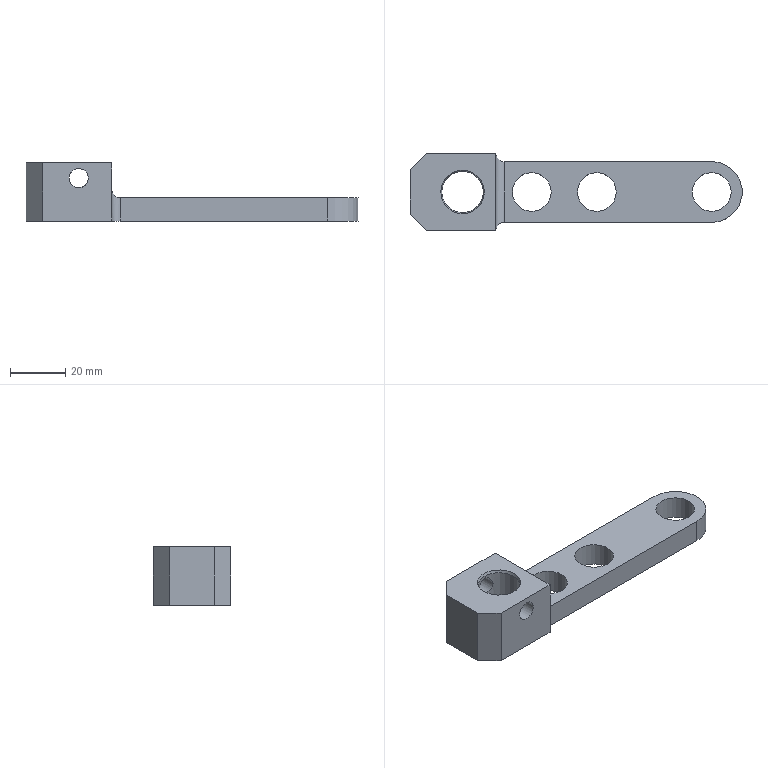NC program | NX | posted with a generic post | part box 120 x 28 x 21 mm
Lines 1651 to 1970 of 1970:
(ZLEVEL_PROFILE_STEEP , TOOL : 5R0.5)
N3246 T07 M6
N3248 G53
N3250 G17 G0 G90 X-41.022 Y-0.016 B0. C0. S4500 M3
N3252 G43 Z20. H7
N3254 Z1.172
N3256 G94 G1 Z0.172 F1000.
N3258 X-43.402 Y-1.627
N3260 G3 X-41.002 Y-4.027 R2.4
N3262 X-36.977 Y-0.003 R4.024
N3264 X-41.002 Y-4.027 R-4.024
N3266 G1 X-40.719 Y-4.002 Z0.157
N3268 X-40.435 Y-3.977 Z0.142
N3270 G3 X-41.002 Y-4.017 R-4.014
N3272 G1 X-40.719 Y-3.991 Z0.127
N3274 X-40.436 Y-3.964 Z0.112
N3276 G3 X-41.002 Y-4.004 R-4.002
N3278 G1 X-40.719 Y-3.98 Z0.097
N3280 X-40.436 Y-3.952 Z0.082
N3282 G3 X-41.002 Y-3.992 R-3.99
N3284 G1 X-40.719 Y-3.969 Z0.067
N3286 X-40.436 Y-3.939 Z0.052
N3288 G3 X-41.002 Y-3.979 R-3.979
N3290 G1 X-40.718 Y-3.959 Z0.037
N3292 X-40.436 Y-3.926 Z0.022
N3294 G3 X-41.002 Y-3.966 R-3.966
N3296 G1 X-40.718 Y-3.948 Z0.007
N3298 X-40.434 Y-3.924 Z-0.007
N3300 G3 X-41.002 Y-3.964 R-3.964
N3302 G1 X-40.719 Y-3.937 Z-0.022
N3304 X-40.437 Y-3.905 Z-0.037
N3306 G3 X-41.002 Y-3.946 R-3.946
N3308 G1 X-40.718 Y-3.926 Z-0.052
N3310 X-40.435 Y-3.896 Z-0.067
N3312 G3 X-41.002 Y-3.936 R-3.936
N3314 G1 X-40.718 Y-3.916 Z-0.082
N3316 X-40.436 Y-3.883 Z-0.097
N3318 G3 X-41.002 Y-3.924 R-3.924
N3320 G1 X-40.718 Y-3.906 Z-0.112
N3322 X-40.436 Y-3.873 Z-0.127
N3324 G3 X-41.002 Y-3.914 R-3.914
N3326 G1 X-40.718 Y-3.896 Z-0.142
N3328 X-40.435 Y-3.863 Z-0.157
N3330 G3 X-41.002 Y-3.904 R-3.904
N3332 G1 X-40.718 Y-3.886 Z-0.172
N3334 X-40.435 Y-3.854 Z-0.187
N3336 G3 X-41.002 Y-3.895 R-3.894
N3338 G1 X-40.718 Y-3.876 Z-0.201
N3340 X-40.436 Y-3.842 Z-0.216
N3342 G3 X-41.002 Y-3.884 R-3.883
N3344 G1 X-40.718 Y-3.867 Z-0.231
N3346 X-40.436 Y-3.833 Z-0.246
N3348 G3 X-41.002 Y-3.874 R-3.873
N3350 G1 X-40.718 Y-3.857 Z-0.261
N3352 X-40.436 Y-3.82 Z-0.276
N3354 G3 X-41.002 Y-3.861 R-3.861
N3356 G1 X-40.718 Y-3.848 Z-0.291
N3358 X-40.436 Y-3.81 Z-0.306
N3360 G3 X-41.002 Y-3.852 R-3.852
N3362 G1 X-40.718 Y-3.838 Z-0.321
N3364 X-40.436 Y-3.8 Z-0.336
N3366 G3 X-41.002 Y-3.842 R-3.842
N3368 G1 X-40.717 Y-3.827 Z-0.351
N3370 X-40.433 Y-3.807 Z-0.366
N3372 G3 X-38.622 Y-3.01 R4.394
N3374 G1 X-38.612 Y-3.021
N3376 G3 X-37.201 Y-0.629 R3.851
N3378 X-37.201 Y0.629 R6.692
N3380 G1 X-37.218 Y0.724
N3382 G3 X-41.357 Y3.837 R3.921
N3384 X-43.396 Y2.996 R4.255
N3386 X-44.6 Y1.289 R3.498
N3388 G1 X-44.783 Y0.721
N3390 X-44.799 Y0.629
N3392 G3 X-44.799 Y-0.629 R5.812
N3394 X-43.393 Y-3.017 R3.851
N3396 G1 X-43.383 Y-3.006
N3398 G3 X-41.002 Y-3.849 R3.987
N3400 G1 X-40.718 Y-3.835 Z-0.381
N3402 X-40.437 Y-3.798 Z-0.396
N3404 G3 X-38.276 Y2.707 R3.84
N3406 G1 X-38.997 Y3.304
N3408 G3 X-40.396 Y3.792 R6.376
N3410 X-43.265 Y3.1 R3.84
N3412 G1 X-43.257 Y3.089
N3414 X-43.347 Y3.022
N3416 G3 X-44.701 Y0.966 R3.747
N3418 G1 X-44.746 Y0.776
N3420 X-44.767 Y0.744
N3422 G3 X-43.385 Y-3.009 R3.84
N3424 G1 X-43.259 Y-3.092
N3426 X-42.982 Y-3.289
N3428 G3 X-41.002 Y-3.84 R3.84
N3430 G1 X-40.718 Y-3.824 Z-0.41
N3432 X-40.436 Y-3.787 Z-0.425
N3434 G3 X-39.161 Y-3.359 R3.829
N3436 G1 X-38.66 Y-3.016
N3438 X-38.626 Y-3.004
N3440 G3 X-37.417 Y-1.352 R3.829
N3442 G1 X-37.243 Y-0.741
N3444 G3 X-38.095 Y2.495 R3.829
N3446 G1 X-38.515 Y2.913
N3448 X-38.59 Y2.976
N3450 X-38.646 Y3.006
N3452 X-38.741 Y3.092
N3454 G3 X-39.655 Y3.585 R3.829
N3456 X-40.398 Y3.782 R28.134
N3458 X-43.259 Y3.092 R3.829
N3460 G1 X-43.276 Y3.064
N3462 X-43.387 Y2.98
N3464 G3 X-44.695 Y0.947 R3.792
N3466 G2 X-44.757 Y0.741 R2.485
N3468 G3 X-43.182 Y-3.146 R3.829
N3470 G1 X-42.283 Y-3.608
N3472 G3 X-41.002 Y-3.829 R3.829
N3474 G1 X-40.718 Y-3.813 Z-0.44
N3476 X-40.436 Y-3.776 Z-0.455
N3478 X-40.382 Y-3.768
N3480 X-40.042 Y-3.666
N3482 X-39.931 Y-3.685
N3484 X-39.214 Y-3.375
N3486 G3 X-37.665 Y-1.859 R3.818
N3488 G1 X-37.346 Y-1.107
N3490 G3 X-37.254 Y0.739 R3.818
N3492 G1 X-37.272 Y0.766
N3494 X-37.36 Y1.154
N3496 G3 X-37.909 Y2.242 R3.818
N3498 G1 X-37.941 Y2.266
N3500 X-38.169 Y2.562
N3502 G3 X-38.388 Y2.785 R3.818
N3504 G1 X-38.522 Y2.905
N3506 G3 X-41.589 Y3.773 R3.818
N3508 G2 X-42.186 Y3.64 R5.818
N3510 G1 X-42.591 Y3.459
N3512 X-42.622 Y3.456
N3514 G3 X-44.647 Y1.131 R3.818
N3516 G1 X-44.681 Y0.961
N3518 G2 X-44.746 Y0.739 R0.894
N3520 G3 X-44.745 Y-0.746 R3.818
N3522 G1 X-44.587 Y-1.309
N3524 G3 X-44.091 Y-2.242 R3.818
N3526 G1 X-44.059 Y-2.266
N3528 X-43.831 Y-2.562
N3530 G3 X-43.614 Y-2.783 R3.818
N3532 G1 X-43.583 Y-2.796
N3534 X-43.472 Y-2.91
N3536 G3 X-42.897 Y-3.314 R3.818
N3538 G1 X-42.236 Y-3.613
N3540 G3 X-41.002 Y-3.818 R3.818
N3542 G1 X-40.718 Y-3.802 Z-0.47
N3544 X-40.436 Y-3.765 Z-0.485
N3546 G3 X-39.905 Y-3.646 R3.807
N3548 G1 X-39.879 Y-3.628
N3550 X-39.504 Y-3.501
N3552 G3 X-37.587 Y-1.687 R3.807
N3554 G1 X-37.356 Y-1.103
N3556 X-37.325 Y-0.995
N3558 X-37.301 Y-0.856
N3560 X-37.264 Y-0.736
N3562 G3 X-37.363 Y1.127 R3.807
N3564 G1 X-37.596 Y1.706
N3566 G3 X-37.909 Y2.223 R3.807
N3568 G1 X-38.004 Y2.332
N3570 X-38.039 Y2.393
N3572 G3 X-39.49 Y3.495 R3.807
N3574 G1 X-39.522 Y3.497
N3576 X-39.878 Y3.627
N3578 X-39.905 Y3.646
N3580 G3 X-42.095 Y3.646 R3.807
N3582 G1 X-42.121 Y3.628
N3584 X-42.496 Y3.501
N3586 G3 X-44.486 Y1.532 R3.807
N3588 G1 X-44.644 Y1.103
N3590 G3 X-44.637 Y-1.127 R3.807
N3592 G1 X-44.404 Y-1.706
N3594 G3 X-44.091 Y-2.223 R3.807
N3596 G1 X-43.996 Y-2.332
N3598 X-43.961 Y-2.393
N3600 G3 X-43.606 Y-2.776 R3.807
N3602 G1 X-43.531 Y-2.83
N3604 X-43.487 Y-2.883
N3606 G3 X-42.891 Y-3.304 R3.807
N3608 G1 X-42.767 Y-3.372
N3610 G3 X-42.51 Y-3.495 R3.807
N3612 G1 X-42.478 Y-3.497
N3614 X-42.122 Y-3.627
N3616 X-42.095 Y-3.646
N3618 X-41.986 Y-3.678
N3620 X-41.945 Y-3.679
N3622 X-41.826 Y-3.706
N3624 X-41.597 Y-3.76
N3626 G3 X-41.002 Y-3.807 R3.807
N3628 G1 X-40.718 Y-3.791 Z-0.5
N3630 X-40.436 Y-3.754 Z-0.515
N3632 G3 X-38.037 Y-2.373 R3.796
N3634 G1 X-38.008 Y-2.319
N3636 X-37.963 Y-2.278
N3638 G3 X-40.002 Y3.663 R3.796
N3640 G2 X-40.405 Y3.75 R1.427
N3642 G3 X-43.983 Y2.349 R3.796
N3644 G1 X-44.056 Y2.252
N3646 G3 X-43.015 Y-3.218 R3.796
N3648 G1 X-42.886 Y-3.295
N3650 G3 X-41.002 Y-3.796 R3.796
N3652 G1 X-40.718 Y-3.781 Z-0.53
N3654 X-40.436 Y-3.743 Z-0.545
N3656 G3 X-38.923 Y-3.165 R3.786
N3658 G1 X-38.679 Y-2.991
N3660 G3 X-43.353 Y-2.965 R-3.786
N3662 G1 X-43.234 Y-3.056
N3664 G3 X-41.002 Y-3.786 R3.786
N3666 G1 X-40.718 Y-3.77 Z-0.56
N3668 X-40.436 Y-3.732 Z-0.575
N3670 G3 X-38.763 Y-3.041 R3.775
N3672 G1 X-38.686 Y-2.982
N3674 G3 X-44.64 Y0.999 R-3.775
N3676 G1 X-44.635 Y0.904
N3678 X-44.704 Y0.729
N3680 G3 X-41.002 Y-3.775 R3.775
N3682 G1 X-40.718 Y-3.759 Z-0.59
N3684 X-40.436 Y-3.721 Z-0.604
N3686 G3 X-41.002 Y-3.764 R-3.764
N3688 G1 X-40.718 Y-3.748 Z-0.619
N3690 X-40.436 Y-3.71 Z-0.634
N3692 G3 X-41.002 Y-3.753 R-3.753
N3694 G1 X-40.718 Y-3.737 Z-0.649
N3696 X-40.436 Y-3.699 Z-0.664
N3698 G3 X-41.002 Y-3.742 R-3.742
N3700 G1 X-40.718 Y-3.726 Z-0.679
N3702 X-40.436 Y-3.688 Z-0.694
N3704 G3 X-41.002 Y-3.731 R-3.731
N3706 G1 X-40.718 Y-3.715 Z-0.709
N3708 X-40.436 Y-3.677 Z-0.724
N3710 G3 X-41.002 Y-3.72 R-3.72
N3712 G1 X-40.718 Y-3.704 Z-0.739
N3714 X-40.436 Y-3.666 Z-0.754
N3716 G3 X-41.002 Y-3.71 R-3.71
N3718 G1 X-40.718 Y-3.693 Z-0.769
N3720 X-40.436 Y-3.655 Z-0.784
N3722 G3 X-41.002 Y-3.699 R-3.699
N3724 G1 X-40.718 Y-3.682 Z-0.799
N3726 X-40.436 Y-3.644 Z-0.813
N3728 G3 X-41.002 Y-3.688 R-3.688
N3730 G1 X-40.718 Y-3.672 Z-0.828
N3732 X-40.436 Y-3.633 Z-0.843
N3734 G3 X-41.002 Y-3.677 R-3.677
N3736 G1 X-40.718 Y-3.661 Z-0.858
N3738 X-40.436 Y-3.622 Z-0.873
N3740 G3 X-41.002 Y-3.666 R-3.666
N3742 G1 X-40.718 Y-3.65 Z-0.888
N3744 X-40.436 Y-3.611 Z-0.903
N3746 G3 X-41.002 Y-3.655 R-3.655
N3748 G1 X-40.718 Y-3.639 Z-0.918
N3750 X-40.436 Y-3.6 Z-0.933
N3752 G3 X-41.002 Y-3.644 R-3.644
N3754 G1 X-40.718 Y-3.628 Z-0.948
N3756 X-40.436 Y-3.589 Z-0.963
N3758 G3 X-41.002 Y-3.633 R-3.633
N3760 G1 X-40.718 Y-3.617 Z-0.978
N3762 X-40.436 Y-3.578 Z-0.993
N3764 G3 X-41.002 Y-3.623 R-3.623
N3766 G1 X-40.718 Y-3.606 Z-1.007
N3768 X-40.436 Y-3.567 Z-1.022
N3770 G3 X-41.002 Y-3.612 R-3.612
N3772 G1 X-40.718 Y-3.595 Z-1.037
N3774 X-40.436 Y-3.556 Z-1.052
N3776 G3 X-41.002 Y-3.601 R-3.601
N3778 G1 X-40.718 Y-3.584 Z-1.067
N3780 X-40.436 Y-3.545 Z-1.082
N3782 G3 X-41.002 Y-3.59 R-3.59
N3784 G1 X-40.718 Y-3.574 Z-1.097
N3786 X-40.436 Y-3.534 Z-1.112
N3788 G3 X-41.002 Y-3.579 R-3.579
N3790 G1 X-40.718 Y-3.563 Z-1.127
N3792 X-40.436 Y-3.523 Z-1.142
N3794 G3 X-41.002 Y-3.568 R-3.568
N3796 G1 X-40.718 Y-3.55 Z-1.157
N3798 X-40.436 Y-3.512 Z-1.172
N3800 G3 X-41.002 Y-3.557 R-3.557
N3802 G1 X-40.718 Y-3.536 Z-1.187
N3804 X-40.436 Y-3.501 Z-1.201
N3806 G3 X-41.002 Y-3.547 R-3.547
N3808 G1 X-40.719 Y-3.523 Z-1.216
N3810 X-40.439 Y-3.473 Z-1.231
N3812 G3 X-41.002 Y-3.518 R-3.518
N3814 G1 X-40.717 Y-3.509 Z-1.246
N3816 X-40.436 Y-3.461 Z-1.261
N3818 G3 X-41.002 Y-3.507 R-3.506
N3820 G1 X-40.718 Y-3.495 Z-1.276
N3822 X-40.436 Y-3.449 Z-1.291
N3824 G3 X-41.002 Y-3.495 R-3.495
N3826 G1 X-40.718 Y-3.482 Z-1.306
N3828 X-40.436 Y-3.438 Z-1.321
N3830 G3 X-41.002 Y-3.483 R-3.484
N3832 G1 X-40.718 Y-3.468 Z-1.336
N3834 X-40.436 Y-3.426 Z-1.351
N3836 G3 X-41.002 Y-3.472 R-3.472
N3838 G1 X-40.718 Y-3.455 Z-1.366
N3840 X-40.436 Y-3.414 Z-1.381
N3842 G3 X-41.002 Y-3.46 R-3.461
N3844 G1 X-40.718 Y-3.441 Z-1.396
N3846 X-40.436 Y-3.402 Z-1.41
N3848 G3 X-41.002 Y-3.449 R-3.449
N3850 G1 X-40.718 Y-3.428 Z-1.425
N3852 X-40.436 Y-3.392 Z-1.44
N3854 G3 X-41.002 Y-3.439 R-3.439
N3856 G1 X-40.719 Y-3.414 Z-1.455
N3858 X-40.436 Y-3.38 Z-1.47
N3860 G3 X-41.002 Y-3.427 R-3.427
N3862 G1 X-40.719 Y-3.403 Z-1.485
N3864 X-40.436 Y-3.369 Z-1.5
N3866 G3 X-37.632 Y0.564 R3.416
N3868 X-40.436 Y-3.369 R-3.416
N3870 X-39.658 Y-2.882 R1.2
N3872 G1 Z-0.5
N3874 G0 Z20.
N3876 M5
N3878 M2